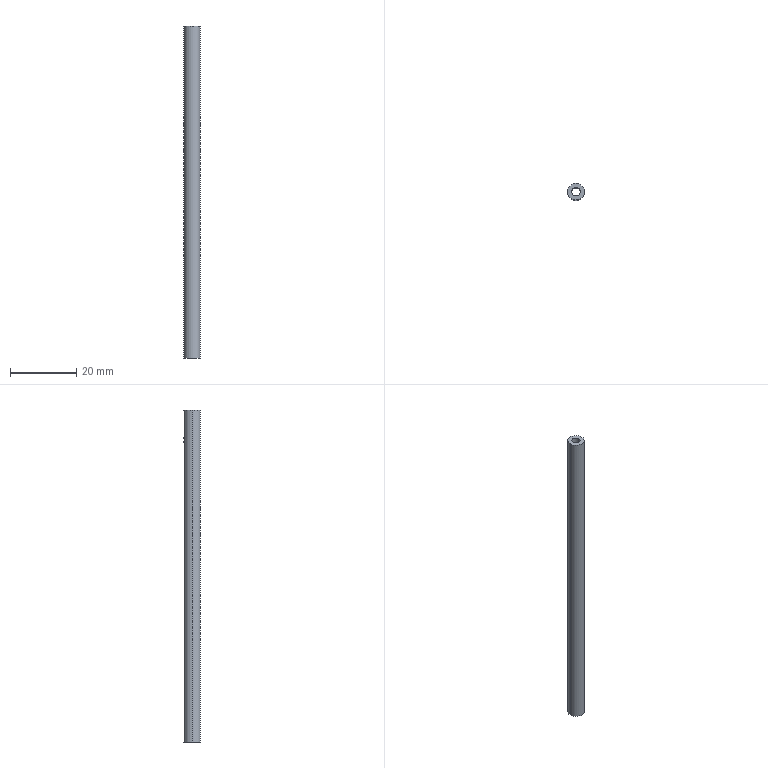Part | SolidWorks | features Extrusion 1, ICE 1 | 1 solid | 8 faces | box 5 x 5 x 100 mm | volume 1470 mm3 | cylinder 6 | plane 2 | commonest cylinder face diameters 1.5 x2 2.5 x2 5 x2
STEP:
#1=CARTESIAN_POINT('',(0.,1.25,90.25));
#2=VERTEX_POINT('',#1);
#3=CARTESIAN_POINT('',(0.,1.25,91.75));
#4=VERTEX_POINT('',#3);
#5=CARTESIAN_POINT('',(0.,1.25,90.25));
#6=CARTESIAN_POINT('',(-0.1013,1.25,90.25));
#7=CARTESIAN_POINT('',(-0.2015,1.237,90.271));
#8=CARTESIAN_POINT('',(-0.3823,1.194,90.347));
#9=CARTESIAN_POINT('',(-0.4637,1.163,90.403));
#10=CARTESIAN_POINT('',(-0.5987,1.1,90.538));
#11=CARTESIAN_POINT('',(-0.6529,1.067,90.618));
#12=CARTESIAN_POINT('',(-0.729,1.016,90.798));
#13=CARTESIAN_POINT('',(-0.75,1.,90.899));
#14=CARTESIAN_POINT('',(-0.75,1.,91.101));
#15=CARTESIAN_POINT('',(-0.7292,1.016,91.201));
#16=CARTESIAN_POINT('',(-0.6534,1.067,91.381));
#17=CARTESIAN_POINT('',(-0.5992,1.1,91.461));
#18=CARTESIAN_POINT('',(-0.4629,1.164,91.598));
#19=CARTESIAN_POINT('',(-0.3828,1.194,91.652));
#20=CARTESIAN_POINT('',(-0.2008,1.237,91.729));
#21=CARTESIAN_POINT('',(-0.1017,1.25,91.75));
#22=CARTESIAN_POINT('',(0.,1.25,91.75));
#23=B_SPLINE_CURVE_WITH_KNOTS('',3,(#5,#6,#7,#8,#9,#10,#11,#12,#13,#14,#15,#16,#17,#18,#19,#20,#21,#22),.UNSPECIFIED.,.F.,.F.,(4,2,2,2,2,2,2,2,4),(0.002406,0.002706,0.003007,0.003307,0.003607,0.003907,0.004207,0.004507,0.004808),.UNSPECIFIED.);
#24=EDGE_CURVE('',#2,#4,#23,.T.);
#25=ORIENTED_EDGE('',*,*,#24,.F.);
#26=CARTESIAN_POINT('',(0.,2.5,90.25));
#27=VERTEX_POINT('',#26);
#28=CARTESIAN_POINT('',(0.,-2.501,90.25));
#29=DIRECTION('',(0.,1.,0.));
#30=VECTOR('',#29,1000.);
#31=LINE('',#28,#30);
#32=EDGE_CURVE('',#2,#27,#31,.T.);
#33=ORIENTED_EDGE('',*,*,#32,.T.);
#34=CARTESIAN_POINT('',(0.,2.5,91.75));
#35=VERTEX_POINT('',#34);
#36=CARTESIAN_POINT('',(0.,2.5,91.75));
#37=CARTESIAN_POINT('',(-0.09973,2.5,91.75));
#38=CARTESIAN_POINT('',(-0.1975,2.494,91.73));
#39=CARTESIAN_POINT('',(-0.379,2.473,91.655));
#40=CARTESIAN_POINT('',(-0.4618,2.458,91.599));
#41=CARTESIAN_POINT('',(-0.5993,2.428,91.461));
#42=CARTESIAN_POINT('',(-0.655,2.413,91.378));
#43=CARTESIAN_POINT('',(-0.73,2.391,91.198));
#44=CARTESIAN_POINT('',(-0.75,2.385,91.099));
#45=CARTESIAN_POINT('',(-0.75,2.385,90.902));
#46=CARTESIAN_POINT('',(-0.7305,2.391,90.803));
#47=CARTESIAN_POINT('',(-0.6547,2.413,90.621));
#48=CARTESIAN_POINT('',(-0.5994,2.428,90.539));
#49=CARTESIAN_POINT('',(-0.4609,2.458,90.4));
#50=CARTESIAN_POINT('',(-0.3782,2.473,90.345));
#51=CARTESIAN_POINT('',(-0.1974,2.494,90.27));
#52=CARTESIAN_POINT('',(-0.09827,2.5,90.25));
#53=CARTESIAN_POINT('',(0.,2.5,90.25));
#54=B_SPLINE_CURVE_WITH_KNOTS('',3,(#36,#37,#38,#39,#40,#41,#42,#43,#44,#45,#46,#47,#48,#49,#50,#51,#52,#53),.UNSPECIFIED.,.F.,.F.,(4,2,2,2,2,2,2,2,4),(0.,0.0002948,0.0005896,0.0008844,0.001179,0.001474,0.001769,0.002064,0.002359),.UNSPECIFIED.);
#55=EDGE_CURVE('',#35,#27,#54,.T.);
#56=ORIENTED_EDGE('',*,*,#55,.F.);
#57=CARTESIAN_POINT('',(0.,-2.501,91.75));
#58=DIRECTION('',(0.,1.,0.));
#59=VECTOR('',#58,1000.);
#60=LINE('',#57,#59);
#61=EDGE_CURVE('',#4,#35,#60,.T.);
#62=ORIENTED_EDGE('',*,*,#61,.F.);
#63=EDGE_LOOP('',(#25,#33,#56,#62));
#64=FACE_OUTER_BOUND('',#63,.T.);
#65=CARTESIAN_POINT('',(0.,-2.501,91.));
#66=DIRECTION('',(0.,1.,0.));
#67=DIRECTION('',(0.,0.,1.));
#68=AXIS2_PLACEMENT_3D('',#65,#66,#67);
#69=CYLINDRICAL_SURFACE('',#68,0.75);
#70=ADVANCED_FACE('',(#64),#69,.F.);
#71=CARTESIAN_POINT('',(-1.25,0.,100.));
#72=VERTEX_POINT('',#71);
#73=CARTESIAN_POINT('',(1.25,0.,100.));
#74=VERTEX_POINT('',#73);
#75=CARTESIAN_POINT('',(0.,0.,100.));
#76=DIRECTION('',(0.,0.,1.));
#77=DIRECTION('',(1.,0.,0.));
#78=AXIS2_PLACEMENT_3D('',#75,#76,#77);
#79=CIRCLE('',#78,1.25);
#80=EDGE_CURVE('',#72,#74,#79,.T.);
#81=ORIENTED_EDGE('',*,*,#80,.T.);
#82=CARTESIAN_POINT('',(1.25,0.,0.));
#83=VERTEX_POINT('',#82);
#84=CARTESIAN_POINT('',(1.25,0.,100.));
#85=DIRECTION('',(0.,0.,-1.));
#86=VECTOR('',#85,1000.);
#87=LINE('',#84,#86);
#88=EDGE_CURVE('',#74,#83,#87,.T.);
#89=ORIENTED_EDGE('',*,*,#88,.T.);
#90=CARTESIAN_POINT('',(-1.25,0.,0.));
#91=VERTEX_POINT('',#90);
#92=CARTESIAN_POINT('',(0.,0.,0.));
#93=DIRECTION('',(0.,0.,1.));
#94=DIRECTION('',(1.,0.,0.));
#95=AXIS2_PLACEMENT_3D('',#92,#93,#94);
#96=CIRCLE('',#95,1.25);
#97=EDGE_CURVE('',#91,#83,#96,.T.);
#98=ORIENTED_EDGE('',*,*,#97,.F.);
#99=CARTESIAN_POINT('',(-1.25,0.,100.));
#100=DIRECTION('',(0.,0.,-1.));
#101=VECTOR('',#100,1000.);
#102=LINE('',#99,#101);
#103=EDGE_CURVE('',#72,#91,#102,.T.);
#104=ORIENTED_EDGE('',*,*,#103,.F.);
#105=EDGE_LOOP('',(#81,#89,#98,#104));
#106=FACE_OUTER_BOUND('',#105,.T.);
#107=CARTESIAN_POINT('',(0.,0.,100.));
#108=DIRECTION('',(0.,0.,-1.));
#109=DIRECTION('',(-1.,0.,0.));
#110=AXIS2_PLACEMENT_3D('',#107,#108,#109);
#111=CYLINDRICAL_SURFACE('',#110,1.25);
#112=ADVANCED_FACE('',(#106),#111,.F.);
#113=ORIENTED_EDGE('',*,*,#55,.T.);
#114=CARTESIAN_POINT('',(0.,2.5,90.25));
#115=CARTESIAN_POINT('',(0.09824,2.5,90.25));
#116=CARTESIAN_POINT('',(0.1974,2.494,90.27));
#117=CARTESIAN_POINT('',(0.3783,2.473,90.345));
#118=CARTESIAN_POINT('',(0.4611,2.458,90.4));
#119=CARTESIAN_POINT('',(0.6687,2.413,90.608));
#120=CARTESIAN_POINT('',(0.75,2.385,90.802));
#121=CARTESIAN_POINT('',(0.75,2.385,91.198));
#122=CARTESIAN_POINT('',(0.668,2.413,91.393));
#123=CARTESIAN_POINT('',(0.3931,2.473,91.668));
#124=CARTESIAN_POINT('',(0.1994,2.5,91.75));
#125=CARTESIAN_POINT('',(0.,2.5,91.75));
#126=B_SPLINE_CURVE_WITH_KNOTS('',3,(#114,#115,#116,#117,#118,#119,#120,#121,#122,#123,#124,#125),.UNSPECIFIED.,.F.,.F.,(4,2,2,2,2,4),(0.002359,0.002653,0.002948,0.003537,0.004127,0.004716),.UNSPECIFIED.);
#127=EDGE_CURVE('',#27,#35,#126,.T.);
#128=ORIENTED_EDGE('',*,*,#127,.T.);
#129=EDGE_LOOP('',(#113,#128));
#130=FACE_BOUND('',#129,.T.);
#131=CARTESIAN_POINT('',(2.5,0.,100.));
#132=VERTEX_POINT('',#131);
#133=CARTESIAN_POINT('',(-2.5,0.,100.));
#134=VERTEX_POINT('',#133);
#135=CARTESIAN_POINT('',(0.,0.,100.));
#136=DIRECTION('',(0.,0.,1.));
#137=DIRECTION('',(1.,0.,0.));
#138=AXIS2_PLACEMENT_3D('',#135,#136,#137);
#139=CIRCLE('',#138,2.5);
#140=EDGE_CURVE('',#132,#134,#139,.T.);
#141=ORIENTED_EDGE('',*,*,#140,.F.);
#142=CARTESIAN_POINT('',(2.5,0.,0.));
#143=VERTEX_POINT('',#142);
#144=CARTESIAN_POINT('',(2.5,0.,100.));
#145=DIRECTION('',(0.,0.,-1.));
#146=VECTOR('',#145,1000.);
#147=LINE('',#144,#146);
#148=EDGE_CURVE('',#132,#143,#147,.T.);
#149=ORIENTED_EDGE('',*,*,#148,.T.);
#150=CARTESIAN_POINT('',(-2.5,0.,0.));
#151=VERTEX_POINT('',#150);
#152=CARTESIAN_POINT('',(0.,0.,0.));
#153=DIRECTION('',(0.,0.,1.));
#154=DIRECTION('',(1.,0.,0.));
#155=AXIS2_PLACEMENT_3D('',#152,#153,#154);
#156=CIRCLE('',#155,2.5);
#157=EDGE_CURVE('',#143,#151,#156,.T.);
#158=ORIENTED_EDGE('',*,*,#157,.T.);
#159=CARTESIAN_POINT('',(-2.5,0.,100.));
#160=DIRECTION('',(0.,0.,-1.));
#161=VECTOR('',#160,1000.);
#162=LINE('',#159,#161);
#163=EDGE_CURVE('',#134,#151,#162,.T.);
#164=ORIENTED_EDGE('',*,*,#163,.F.);
#165=EDGE_LOOP('',(#141,#149,#158,#164));
#166=FACE_OUTER_BOUND('',#165,.T.);
#167=CARTESIAN_POINT('',(0.,0.,100.));
#168=DIRECTION('',(0.,0.,-1.));
#169=DIRECTION('',(-1.,0.,0.));
#170=AXIS2_PLACEMENT_3D('',#167,#168,#169);
#171=CYLINDRICAL_SURFACE('',#170,2.5);
#172=ADVANCED_FACE('',(#130,#166),#171,.T.);
#173=CARTESIAN_POINT('',(0.,0.,100.));
#174=DIRECTION('',(0.,0.,1.));
#175=DIRECTION('',(1.,0.,0.));
#176=AXIS2_PLACEMENT_3D('',#173,#174,#175);
#177=CIRCLE('',#176,2.5);
#178=EDGE_CURVE('',#134,#132,#177,.T.);
#179=ORIENTED_EDGE('',*,*,#178,.T.);
#180=ORIENTED_EDGE('',*,*,#140,.T.);
#181=EDGE_LOOP('',(#179,#180));
#182=FACE_OUTER_BOUND('',#181,.T.);
#183=ORIENTED_EDGE('',*,*,#80,.F.);
#184=CARTESIAN_POINT('',(0.,0.,100.));
#185=DIRECTION('',(0.,0.,1.));
#186=DIRECTION('',(1.,0.,0.));
#187=AXIS2_PLACEMENT_3D('',#184,#185,#186);
#188=CIRCLE('',#187,1.25);
#189=EDGE_CURVE('',#74,#72,#188,.T.);
#190=ORIENTED_EDGE('',*,*,#189,.F.);
#191=EDGE_LOOP('',(#183,#190));
#192=FACE_BOUND('',#191,.T.);
#193=CARTESIAN_POINT('',(0.,0.,100.));
#194=DIRECTION('',(0.,0.,1.));
#195=DIRECTION('',(1.,0.,0.));
#196=AXIS2_PLACEMENT_3D('',#193,#194,#195);
#197=PLANE('',#196);
#198=ADVANCED_FACE('',(#182,#192),#197,.T.);
#199=CARTESIAN_POINT('',(0.,0.,0.));
#200=DIRECTION('',(0.,0.,1.));
#201=DIRECTION('',(1.,0.,0.));
#202=AXIS2_PLACEMENT_3D('',#199,#200,#201);
#203=CIRCLE('',#202,2.5);
#204=EDGE_CURVE('',#151,#143,#203,.T.);
#205=ORIENTED_EDGE('',*,*,#204,.F.);
#206=ORIENTED_EDGE('',*,*,#157,.F.);
#207=EDGE_LOOP('',(#205,#206));
#208=FACE_OUTER_BOUND('',#207,.T.);
#209=ORIENTED_EDGE('',*,*,#97,.T.);
#210=CARTESIAN_POINT('',(0.,0.,0.));
#211=DIRECTION('',(0.,0.,1.));
#212=DIRECTION('',(1.,0.,0.));
#213=AXIS2_PLACEMENT_3D('',#210,#211,#212);
#214=CIRCLE('',#213,1.25);
#215=EDGE_CURVE('',#83,#91,#214,.T.);
#216=ORIENTED_EDGE('',*,*,#215,.T.);
#217=EDGE_LOOP('',(#209,#216));
#218=FACE_BOUND('',#217,.T.);
#219=CARTESIAN_POINT('',(0.,0.,0.));
#220=DIRECTION('',(0.,0.,1.));
#221=DIRECTION('',(1.,0.,0.));
#222=AXIS2_PLACEMENT_3D('',#219,#220,#221);
#223=PLANE('',#222);
#224=ADVANCED_FACE('',(#208,#218),#223,.F.);
#225=ORIENTED_EDGE('',*,*,#148,.F.);
#226=ORIENTED_EDGE('',*,*,#178,.F.);
#227=ORIENTED_EDGE('',*,*,#163,.T.);
#228=ORIENTED_EDGE('',*,*,#204,.T.);
#229=EDGE_LOOP('',(#225,#226,#227,#228));
#230=FACE_OUTER_BOUND('',#229,.T.);
#231=CARTESIAN_POINT('',(0.,0.,100.));
#232=DIRECTION('',(0.,0.,-1.));
#233=DIRECTION('',(-1.,0.,0.));
#234=AXIS2_PLACEMENT_3D('',#231,#232,#233);
#235=CYLINDRICAL_SURFACE('',#234,2.5);
#236=ADVANCED_FACE('',(#230),#235,.T.);
#237=ORIENTED_EDGE('',*,*,#88,.F.);
#238=ORIENTED_EDGE('',*,*,#189,.T.);
#239=ORIENTED_EDGE('',*,*,#103,.T.);
#240=ORIENTED_EDGE('',*,*,#215,.F.);
#241=EDGE_LOOP('',(#237,#238,#239,#240));
#242=FACE_OUTER_BOUND('',#241,.T.);
#243=CARTESIAN_POINT('',(0.,1.25,91.75));
#244=CARTESIAN_POINT('',(0.1019,1.25,91.75));
#245=CARTESIAN_POINT('',(0.2015,1.237,91.729));
#246=CARTESIAN_POINT('',(0.3826,1.194,91.653));
#247=CARTESIAN_POINT('',(0.4639,1.163,91.597));
#248=CARTESIAN_POINT('',(0.5986,1.1,91.462));
#249=CARTESIAN_POINT('',(0.6532,1.067,91.381));
#250=CARTESIAN_POINT('',(0.7288,1.017,91.202));
#251=CARTESIAN_POINT('',(0.75,1.,91.102));
#252=CARTESIAN_POINT('',(0.75,1.,90.899));
#253=CARTESIAN_POINT('',(0.7291,1.016,90.799));
#254=CARTESIAN_POINT('',(0.6533,1.067,90.619));
#255=CARTESIAN_POINT('',(0.5987,1.1,90.538));
#256=CARTESIAN_POINT('',(0.4632,1.163,90.402));
#257=CARTESIAN_POINT('',(0.3831,1.194,90.348));
#258=CARTESIAN_POINT('',(0.2007,1.237,90.271));
#259=CARTESIAN_POINT('',(0.1015,1.25,90.25));
#260=CARTESIAN_POINT('',(0.,1.25,90.25));
#261=B_SPLINE_CURVE_WITH_KNOTS('',3,(#243,#244,#245,#246,#247,#248,#249,#250,#251,#252,#253,#254,#255,#256,#257,#258,#259,#260),.UNSPECIFIED.,.F.,.F.,(4,2,2,2,2,2,2,2,4),(0.,0.0003008,0.0006015,0.0009023,0.001203,0.001504,0.001805,0.002105,0.002406),.UNSPECIFIED.);
#262=EDGE_CURVE('',#4,#2,#261,.T.);
#263=ORIENTED_EDGE('',*,*,#262,.T.);
#264=ORIENTED_EDGE('',*,*,#24,.T.);
#265=EDGE_LOOP('',(#263,#264));
#266=FACE_BOUND('',#265,.T.);
#267=CARTESIAN_POINT('',(0.,0.,100.));
#268=DIRECTION('',(0.,0.,-1.));
#269=DIRECTION('',(-1.,0.,0.));
#270=AXIS2_PLACEMENT_3D('',#267,#268,#269);
#271=CYLINDRICAL_SURFACE('',#270,1.25);
#272=ADVANCED_FACE('',(#242,#266),#271,.F.);
#273=ORIENTED_EDGE('',*,*,#32,.F.);
#274=ORIENTED_EDGE('',*,*,#262,.F.);
#275=ORIENTED_EDGE('',*,*,#61,.T.);
#276=ORIENTED_EDGE('',*,*,#127,.F.);
#277=EDGE_LOOP('',(#273,#274,#275,#276));
#278=FACE_OUTER_BOUND('',#277,.T.);
#279=CARTESIAN_POINT('',(0.,-2.501,91.));
#280=DIRECTION('',(0.,1.,0.));
#281=DIRECTION('',(0.,0.,1.));
#282=AXIS2_PLACEMENT_3D('',#279,#280,#281);
#283=CYLINDRICAL_SURFACE('',#282,0.75);
#284=ADVANCED_FACE('',(#278),#283,.F.);
#285=CLOSED_SHELL('',(#70,#112,#172,#198,#224,#236,#272,#284));
#286=MANIFOLD_SOLID_BREP('',#285);
#287=CARTESIAN_POINT('',(0.,0.,0.));
#288=DIRECTION('',(0.,0.,1.));
#289=DIRECTION('',(1.,0.,0.));
#290=AXIS2_PLACEMENT_3D('',#287,#288,#289);
#291=(LENGTH_UNIT()NAMED_UNIT(*)SI_UNIT(.MILLI.,.METRE.));
#292=UNCERTAINTY_MEASURE_WITH_UNIT(LENGTH_MEASURE(0.00001),#291,'','');
#293=(NAMED_UNIT(*)PLANE_ANGLE_UNIT()SI_UNIT($,.RADIAN.));
#294=(NAMED_UNIT(*)SI_UNIT($,.STERADIAN.)SOLID_ANGLE_UNIT());
#295=(GEOMETRIC_REPRESENTATION_CONTEXT(3)GLOBAL_UNCERTAINTY_ASSIGNED_CONTEXT((#292))GLOBAL_UNIT_ASSIGNED_CONTEXT((#291,#293,#294))REPRESENTATION_CONTEXT('',''));
#296=ADVANCED_BREP_SHAPE_REPRESENTATION('',(#286,#290),#295);